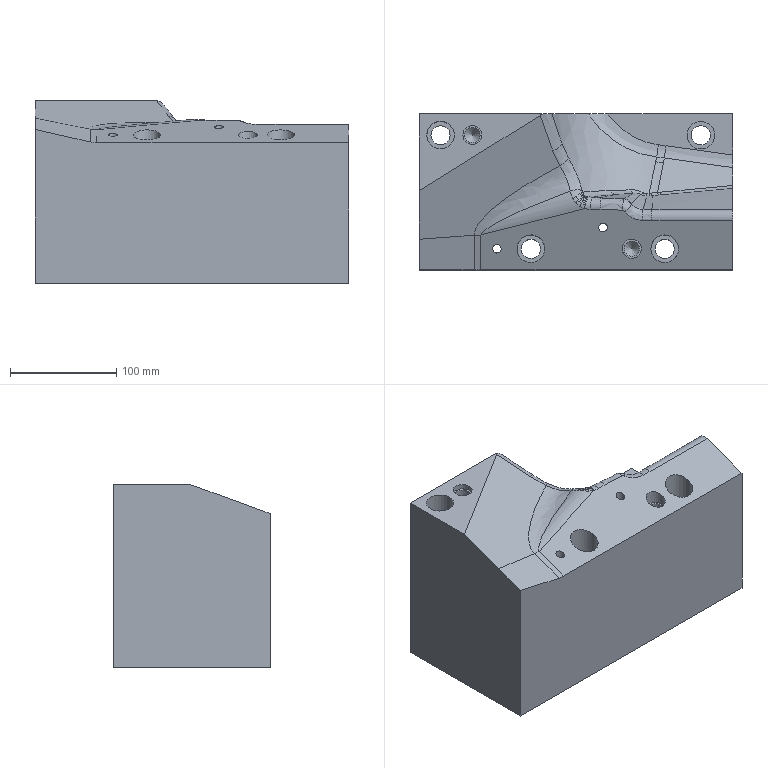Part | STEP file | lll_id78_x_t | 1 solid | 135 faces | box 295 x 147 x 172 mm | volume 5377374 mm3 | spline 69 | cylinder 31 | plane 27 | torus 6 | cone 2 | commonest cylinder face diameters 2 x6 25 x6 18.009 x4 26.008 x4 8.1 x2 12.5 x2